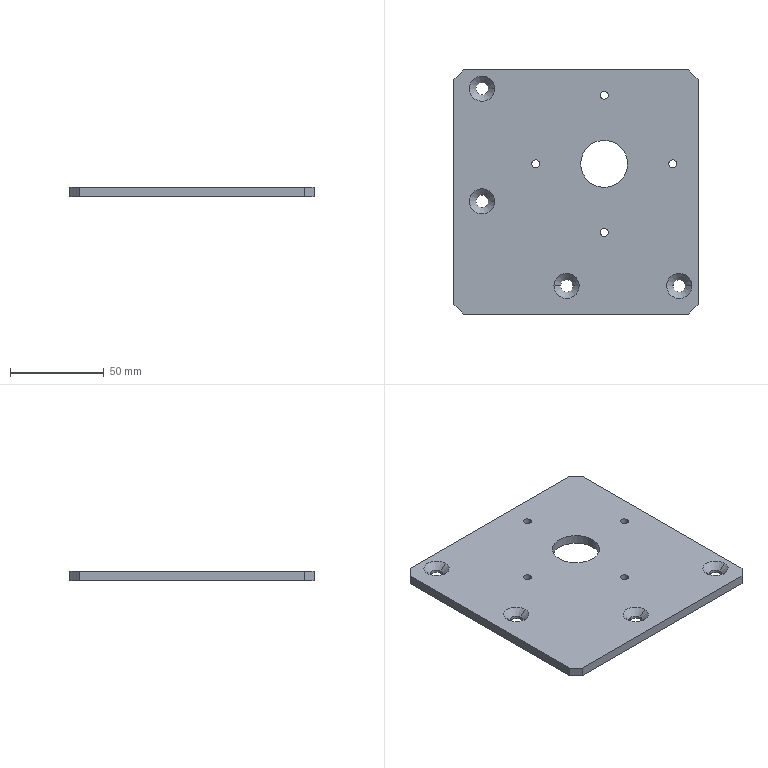Part | SolidWorks | features BaseBody 1 | 1 solid | 36 faces | box 130 x 130 x 5 mm | volume 80182 mm3 | cylinder 18 | plane 10 | cone 8 | commonest cylinder face diameters 4.2 x8 6.6 x8 25 x2
STEP:
#1=CARTESIAN_POINT('',(114.4,80.,0.));
#2=VERTEX_POINT('',#1);
#3=CARTESIAN_POINT('',(118.6,80.,0.));
#4=VERTEX_POINT('',#3);
#5=CARTESIAN_POINT('',(116.5,80.,0.));
#6=DIRECTION('',(0.,0.,1.));
#7=DIRECTION('',(1.,0.,0.));
#8=AXIS2_PLACEMENT_3D('',#5,#6,#7);
#9=CIRCLE('',#8,2.1);
#10=EDGE_CURVE('',#2,#4,#9,.T.);
#11=ORIENTED_EDGE('',*,*,#10,.F.);
#12=CARTESIAN_POINT('',(114.4,80.,5.));
#13=VERTEX_POINT('',#12);
#14=CARTESIAN_POINT('',(114.4,80.,5.));
#15=DIRECTION('',(0.,0.,1.));
#16=VECTOR('',#15,1000.);
#17=LINE('',#14,#16);
#18=EDGE_CURVE('',#2,#13,#17,.T.);
#19=ORIENTED_EDGE('',*,*,#18,.T.);
#20=CARTESIAN_POINT('',(118.6,80.,5.));
#21=VERTEX_POINT('',#20);
#22=CARTESIAN_POINT('',(116.5,80.,5.));
#23=DIRECTION('',(0.,0.,1.));
#24=DIRECTION('',(1.,0.,0.));
#25=AXIS2_PLACEMENT_3D('',#22,#23,#24);
#26=CIRCLE('',#25,2.1);
#27=EDGE_CURVE('',#13,#21,#26,.T.);
#28=ORIENTED_EDGE('',*,*,#27,.T.);
#29=CARTESIAN_POINT('',(118.6,80.,5.));
#30=DIRECTION('',(0.,0.,1.));
#31=VECTOR('',#30,1000.);
#32=LINE('',#29,#31);
#33=EDGE_CURVE('',#4,#21,#32,.T.);
#34=ORIENTED_EDGE('',*,*,#33,.F.);
#35=EDGE_LOOP('',(#11,#19,#28,#34));
#36=FACE_OUTER_BOUND('',#35,.T.);
#37=CARTESIAN_POINT('',(116.5,80.,5.));
#38=DIRECTION('',(0.,0.,1.));
#39=DIRECTION('',(1.,0.,0.));
#40=AXIS2_PLACEMENT_3D('',#37,#38,#39);
#41=CYLINDRICAL_SURFACE('',#40,2.1);
#42=ADVANCED_FACE('',(#36),#41,.F.);
#43=CARTESIAN_POINT('',(77.9,43.5,0.));
#44=VERTEX_POINT('',#43);
#45=CARTESIAN_POINT('',(82.1,43.5,0.));
#46=VERTEX_POINT('',#45);
#47=CARTESIAN_POINT('',(80.,43.5,0.));
#48=DIRECTION('',(0.,0.,1.));
#49=DIRECTION('',(1.,0.,0.));
#50=AXIS2_PLACEMENT_3D('',#47,#48,#49);
#51=CIRCLE('',#50,2.1);
#52=EDGE_CURVE('',#44,#46,#51,.T.);
#53=ORIENTED_EDGE('',*,*,#52,.F.);
#54=CARTESIAN_POINT('',(77.9,43.5,5.));
#55=VERTEX_POINT('',#54);
#56=CARTESIAN_POINT('',(77.9,43.5,5.));
#57=DIRECTION('',(0.,0.,1.));
#58=VECTOR('',#57,1000.);
#59=LINE('',#56,#58);
#60=EDGE_CURVE('',#44,#55,#59,.T.);
#61=ORIENTED_EDGE('',*,*,#60,.T.);
#62=CARTESIAN_POINT('',(82.1,43.5,5.));
#63=VERTEX_POINT('',#62);
#64=CARTESIAN_POINT('',(80.,43.5,5.));
#65=DIRECTION('',(0.,0.,1.));
#66=DIRECTION('',(1.,0.,0.));
#67=AXIS2_PLACEMENT_3D('',#64,#65,#66);
#68=CIRCLE('',#67,2.1);
#69=EDGE_CURVE('',#55,#63,#68,.T.);
#70=ORIENTED_EDGE('',*,*,#69,.T.);
#71=CARTESIAN_POINT('',(82.1,43.5,5.));
#72=DIRECTION('',(0.,0.,1.));
#73=VECTOR('',#72,1000.);
#74=LINE('',#71,#73);
#75=EDGE_CURVE('',#46,#63,#74,.T.);
#76=ORIENTED_EDGE('',*,*,#75,.F.);
#77=EDGE_LOOP('',(#53,#61,#70,#76));
#78=FACE_OUTER_BOUND('',#77,.T.);
#79=CARTESIAN_POINT('',(80.,43.5,5.));
#80=DIRECTION('',(0.,0.,1.));
#81=DIRECTION('',(1.,0.,0.));
#82=AXIS2_PLACEMENT_3D('',#79,#80,#81);
#83=CYLINDRICAL_SURFACE('',#82,2.1);
#84=ADVANCED_FACE('',(#78),#83,.F.);
#85=CARTESIAN_POINT('',(41.4,80.,0.));
#86=VERTEX_POINT('',#85);
#87=CARTESIAN_POINT('',(45.6,80.,0.));
#88=VERTEX_POINT('',#87);
#89=CARTESIAN_POINT('',(43.5,80.,0.));
#90=DIRECTION('',(0.,0.,1.));
#91=DIRECTION('',(1.,0.,0.));
#92=AXIS2_PLACEMENT_3D('',#89,#90,#91);
#93=CIRCLE('',#92,2.1);
#94=EDGE_CURVE('',#86,#88,#93,.T.);
#95=ORIENTED_EDGE('',*,*,#94,.F.);
#96=CARTESIAN_POINT('',(41.4,80.,5.));
#97=VERTEX_POINT('',#96);
#98=CARTESIAN_POINT('',(41.4,80.,5.));
#99=DIRECTION('',(0.,0.,1.));
#100=VECTOR('',#99,1000.);
#101=LINE('',#98,#100);
#102=EDGE_CURVE('',#86,#97,#101,.T.);
#103=ORIENTED_EDGE('',*,*,#102,.T.);
#104=CARTESIAN_POINT('',(45.6,80.,5.));
#105=VERTEX_POINT('',#104);
#106=CARTESIAN_POINT('',(43.5,80.,5.));
#107=DIRECTION('',(0.,0.,1.));
#108=DIRECTION('',(1.,0.,0.));
#109=AXIS2_PLACEMENT_3D('',#106,#107,#108);
#110=CIRCLE('',#109,2.1);
#111=EDGE_CURVE('',#97,#105,#110,.T.);
#112=ORIENTED_EDGE('',*,*,#111,.T.);
#113=CARTESIAN_POINT('',(45.6,80.,5.));
#114=DIRECTION('',(0.,0.,1.));
#115=VECTOR('',#114,1000.);
#116=LINE('',#113,#115);
#117=EDGE_CURVE('',#88,#105,#116,.T.);
#118=ORIENTED_EDGE('',*,*,#117,.F.);
#119=EDGE_LOOP('',(#95,#103,#112,#118));
#120=FACE_OUTER_BOUND('',#119,.T.);
#121=CARTESIAN_POINT('',(43.5,80.,5.));
#122=DIRECTION('',(0.,0.,1.));
#123=DIRECTION('',(1.,0.,0.));
#124=AXIS2_PLACEMENT_3D('',#121,#122,#123);
#125=CYLINDRICAL_SURFACE('',#124,2.1);
#126=ADVANCED_FACE('',(#120),#125,.F.);
#127=CARTESIAN_POINT('',(77.9,116.5,0.));
#128=VERTEX_POINT('',#127);
#129=CARTESIAN_POINT('',(82.1,116.5,0.));
#130=VERTEX_POINT('',#129);
#131=CARTESIAN_POINT('',(80.,116.5,0.));
#132=DIRECTION('',(0.,0.,1.));
#133=DIRECTION('',(1.,0.,0.));
#134=AXIS2_PLACEMENT_3D('',#131,#132,#133);
#135=CIRCLE('',#134,2.1);
#136=EDGE_CURVE('',#128,#130,#135,.T.);
#137=ORIENTED_EDGE('',*,*,#136,.F.);
#138=CARTESIAN_POINT('',(77.9,116.5,5.));
#139=VERTEX_POINT('',#138);
#140=CARTESIAN_POINT('',(77.9,116.5,5.));
#141=DIRECTION('',(0.,0.,1.));
#142=VECTOR('',#141,1000.);
#143=LINE('',#140,#142);
#144=EDGE_CURVE('',#128,#139,#143,.T.);
#145=ORIENTED_EDGE('',*,*,#144,.T.);
#146=CARTESIAN_POINT('',(82.1,116.5,5.));
#147=VERTEX_POINT('',#146);
#148=CARTESIAN_POINT('',(80.,116.5,5.));
#149=DIRECTION('',(0.,0.,1.));
#150=DIRECTION('',(1.,0.,0.));
#151=AXIS2_PLACEMENT_3D('',#148,#149,#150);
#152=CIRCLE('',#151,2.1);
#153=EDGE_CURVE('',#139,#147,#152,.T.);
#154=ORIENTED_EDGE('',*,*,#153,.T.);
#155=CARTESIAN_POINT('',(82.1,116.5,5.));
#156=DIRECTION('',(0.,0.,1.));
#157=VECTOR('',#156,1000.);
#158=LINE('',#155,#157);
#159=EDGE_CURVE('',#130,#147,#158,.T.);
#160=ORIENTED_EDGE('',*,*,#159,.F.);
#161=EDGE_LOOP('',(#137,#145,#154,#160));
#162=FACE_OUTER_BOUND('',#161,.T.);
#163=CARTESIAN_POINT('',(80.,116.5,5.));
#164=DIRECTION('',(0.,0.,1.));
#165=DIRECTION('',(1.,0.,0.));
#166=AXIS2_PLACEMENT_3D('',#163,#164,#165);
#167=CYLINDRICAL_SURFACE('',#166,2.1);
#168=ADVANCED_FACE('',(#162),#167,.F.);
#169=CARTESIAN_POINT('',(67.5,80.,0.));
#170=VERTEX_POINT('',#169);
#171=CARTESIAN_POINT('',(92.5,80.,0.));
#172=VERTEX_POINT('',#171);
#173=CARTESIAN_POINT('',(80.,80.,0.));
#174=DIRECTION('',(0.,0.,1.));
#175=DIRECTION('',(1.,0.,0.));
#176=AXIS2_PLACEMENT_3D('',#173,#174,#175);
#177=CIRCLE('',#176,12.5);
#178=EDGE_CURVE('',#170,#172,#177,.T.);
#179=ORIENTED_EDGE('',*,*,#178,.F.);
#180=CARTESIAN_POINT('',(67.5,80.,5.));
#181=VERTEX_POINT('',#180);
#182=CARTESIAN_POINT('',(67.5,80.,0.));
#183=DIRECTION('',(0.,0.,1.));
#184=VECTOR('',#183,1000.);
#185=LINE('',#182,#184);
#186=EDGE_CURVE('',#170,#181,#185,.T.);
#187=ORIENTED_EDGE('',*,*,#186,.T.);
#188=CARTESIAN_POINT('',(92.5,80.,5.));
#189=VERTEX_POINT('',#188);
#190=CARTESIAN_POINT('',(80.,80.,5.));
#191=DIRECTION('',(0.,0.,1.));
#192=DIRECTION('',(1.,0.,0.));
#193=AXIS2_PLACEMENT_3D('',#190,#191,#192);
#194=CIRCLE('',#193,12.5);
#195=EDGE_CURVE('',#181,#189,#194,.T.);
#196=ORIENTED_EDGE('',*,*,#195,.T.);
#197=CARTESIAN_POINT('',(92.5,80.,0.));
#198=DIRECTION('',(0.,0.,1.));
#199=VECTOR('',#198,1000.);
#200=LINE('',#197,#199);
#201=EDGE_CURVE('',#172,#189,#200,.T.);
#202=ORIENTED_EDGE('',*,*,#201,.F.);
#203=EDGE_LOOP('',(#179,#187,#196,#202));
#204=FACE_OUTER_BOUND('',#203,.T.);
#205=CARTESIAN_POINT('',(80.,80.,0.));
#206=DIRECTION('',(0.,0.,1.));
#207=DIRECTION('',(1.,0.,0.));
#208=AXIS2_PLACEMENT_3D('',#205,#206,#207);
#209=CYLINDRICAL_SURFACE('',#208,12.5);
#210=ADVANCED_FACE('',(#204),#209,.F.);
#211=CARTESIAN_POINT('',(11.7,60.,1.58));
#212=VERTEX_POINT('',#211);
#213=CARTESIAN_POINT('',(18.3,60.,1.58));
#214=VERTEX_POINT('',#213);
#215=CARTESIAN_POINT('',(15.,60.,1.58));
#216=DIRECTION('',(0.,0.,1.));
#217=DIRECTION('',(1.,0.,0.));
#218=AXIS2_PLACEMENT_3D('',#215,#216,#217);
#219=CIRCLE('',#218,3.3);
#220=EDGE_CURVE('',#212,#214,#219,.T.);
#221=ORIENTED_EDGE('',*,*,#220,.F.);
#222=CARTESIAN_POINT('',(8.28,60.,5.));
#223=VERTEX_POINT('',#222);
#224=CARTESIAN_POINT('',(8.28,60.,5.));
#225=DIRECTION('',(-0.7071,0.,0.7071));
#226=VECTOR('',#225,1000.);
#227=LINE('',#224,#226);
#228=EDGE_CURVE('',#212,#223,#227,.T.);
#229=ORIENTED_EDGE('',*,*,#228,.T.);
#230=CARTESIAN_POINT('',(21.72,60.,5.));
#231=VERTEX_POINT('',#230);
#232=CARTESIAN_POINT('',(15.,60.,5.));
#233=DIRECTION('',(0.,0.,1.));
#234=DIRECTION('',(1.,0.,0.));
#235=AXIS2_PLACEMENT_3D('',#232,#233,#234);
#236=CIRCLE('',#235,6.72);
#237=EDGE_CURVE('',#223,#231,#236,.T.);
#238=ORIENTED_EDGE('',*,*,#237,.T.);
#239=CARTESIAN_POINT('',(21.72,60.,5.));
#240=DIRECTION('',(0.7071,0.,0.7071));
#241=VECTOR('',#240,1000.);
#242=LINE('',#239,#241);
#243=EDGE_CURVE('',#214,#231,#242,.T.);
#244=ORIENTED_EDGE('',*,*,#243,.F.);
#245=EDGE_LOOP('',(#221,#229,#238,#244));
#246=FACE_OUTER_BOUND('',#245,.T.);
#247=CARTESIAN_POINT('',(15.,60.,5.));
#248=DIRECTION('',(0.,0.,1.));
#249=DIRECTION('',(1.,0.,0.));
#250=AXIS2_PLACEMENT_3D('',#247,#248,#249);
#251=CONICAL_SURFACE('',#250,6.72,0.7854);
#252=ADVANCED_FACE('',(#246),#251,.F.);
#253=CARTESIAN_POINT('',(11.7,60.,0.));
#254=VERTEX_POINT('',#253);
#255=CARTESIAN_POINT('',(18.3,60.,0.));
#256=VERTEX_POINT('',#255);
#257=CARTESIAN_POINT('',(15.,60.,0.));
#258=DIRECTION('',(0.,0.,1.));
#259=DIRECTION('',(1.,0.,0.));
#260=AXIS2_PLACEMENT_3D('',#257,#258,#259);
#261=CIRCLE('',#260,3.3);
#262=EDGE_CURVE('',#254,#256,#261,.T.);
#263=ORIENTED_EDGE('',*,*,#262,.F.);
#264=CARTESIAN_POINT('',(11.7,60.,5.));
#265=DIRECTION('',(0.,0.,1.));
#266=VECTOR('',#265,1000.);
#267=LINE('',#264,#266);
#268=EDGE_CURVE('',#254,#212,#267,.T.);
#269=ORIENTED_EDGE('',*,*,#268,.T.);
#270=ORIENTED_EDGE('',*,*,#220,.T.);
#271=CARTESIAN_POINT('',(18.3,60.,5.));
#272=DIRECTION('',(0.,0.,1.));
#273=VECTOR('',#272,1000.);
#274=LINE('',#271,#273);
#275=EDGE_CURVE('',#256,#214,#274,.T.);
#276=ORIENTED_EDGE('',*,*,#275,.F.);
#277=EDGE_LOOP('',(#263,#269,#270,#276));
#278=FACE_OUTER_BOUND('',#277,.T.);
#279=CARTESIAN_POINT('',(15.,60.,5.));
#280=DIRECTION('',(0.,0.,1.));
#281=DIRECTION('',(1.,0.,0.));
#282=AXIS2_PLACEMENT_3D('',#279,#280,#281);
#283=CYLINDRICAL_SURFACE('',#282,3.3);
#284=ADVANCED_FACE('',(#278),#283,.F.);
#285=CARTESIAN_POINT('',(11.7,120.,1.58));
#286=VERTEX_POINT('',#285);
#287=CARTESIAN_POINT('',(18.3,120.,1.58));
#288=VERTEX_POINT('',#287);
#289=CARTESIAN_POINT('',(15.,120.,1.58));
#290=DIRECTION('',(0.,0.,1.));
#291=DIRECTION('',(1.,0.,0.));
#292=AXIS2_PLACEMENT_3D('',#289,#290,#291);
#293=CIRCLE('',#292,3.3);
#294=EDGE_CURVE('',#286,#288,#293,.T.);
#295=ORIENTED_EDGE('',*,*,#294,.F.);
#296=CARTESIAN_POINT('',(8.28,120.,5.));
#297=VERTEX_POINT('',#296);
#298=CARTESIAN_POINT('',(8.28,120.,5.));
#299=DIRECTION('',(-0.7071,0.,0.7071));
#300=VECTOR('',#299,1000.);
#301=LINE('',#298,#300);
#302=EDGE_CURVE('',#286,#297,#301,.T.);
#303=ORIENTED_EDGE('',*,*,#302,.T.);
#304=CARTESIAN_POINT('',(21.72,120.,5.));
#305=VERTEX_POINT('',#304);
#306=CARTESIAN_POINT('',(15.,120.,5.));
#307=DIRECTION('',(0.,0.,1.));
#308=DIRECTION('',(1.,0.,0.));
#309=AXIS2_PLACEMENT_3D('',#306,#307,#308);
#310=CIRCLE('',#309,6.72);
#311=EDGE_CURVE('',#297,#305,#310,.T.);
#312=ORIENTED_EDGE('',*,*,#311,.T.);
#313=CARTESIAN_POINT('',(21.72,120.,5.));
#314=DIRECTION('',(0.7071,0.,0.7071));
#315=VECTOR('',#314,1000.);
#316=LINE('',#313,#315);
#317=EDGE_CURVE('',#288,#305,#316,.T.);
#318=ORIENTED_EDGE('',*,*,#317,.F.);
#319=EDGE_LOOP('',(#295,#303,#312,#318));
#320=FACE_OUTER_BOUND('',#319,.T.);
#321=CARTESIAN_POINT('',(15.,120.,5.));
#322=DIRECTION('',(0.,0.,1.));
#323=DIRECTION('',(1.,0.,0.));
#324=AXIS2_PLACEMENT_3D('',#321,#322,#323);
#325=CONICAL_SURFACE('',#324,6.72,0.7854);
#326=ADVANCED_FACE('',(#320),#325,.F.);
#327=CARTESIAN_POINT('',(11.7,120.,0.));
#328=VERTEX_POINT('',#327);
#329=CARTESIAN_POINT('',(18.3,120.,0.));
#330=VERTEX_POINT('',#329);
#331=CARTESIAN_POINT('',(15.,120.,0.));
#332=DIRECTION('',(0.,0.,1.));
#333=DIRECTION('',(1.,0.,0.));
#334=AXIS2_PLACEMENT_3D('',#331,#332,#333);
#335=CIRCLE('',#334,3.3);
#336=EDGE_CURVE('',#328,#330,#335,.T.);
#337=ORIENTED_EDGE('',*,*,#336,.F.);
#338=CARTESIAN_POINT('',(11.7,120.,5.));
#339=DIRECTION('',(0.,0.,1.));
#340=VECTOR('',#339,1000.);
#341=LINE('',#338,#340);
#342=EDGE_CURVE('',#328,#286,#341,.T.);
#343=ORIENTED_EDGE('',*,*,#342,.T.);
#344=ORIENTED_EDGE('',*,*,#294,.T.);
#345=CARTESIAN_POINT('',(18.3,120.,5.));
#346=DIRECTION('',(0.,0.,1.));
#347=VECTOR('',#346,1000.);
#348=LINE('',#345,#347);
#349=EDGE_CURVE('',#330,#288,#348,.T.);
#350=ORIENTED_EDGE('',*,*,#349,.F.);
#351=EDGE_LOOP('',(#337,#343,#344,#350));
#352=FACE_OUTER_BOUND('',#351,.T.);
#353=CARTESIAN_POINT('',(15.,120.,5.));
#354=DIRECTION('',(0.,0.,1.));
#355=DIRECTION('',(1.,0.,0.));
#356=AXIS2_PLACEMENT_3D('',#353,#354,#355);
#357=CYLINDRICAL_SURFACE('',#356,3.3);
#358=ADVANCED_FACE('',(#352),#357,.F.);
#359=CARTESIAN_POINT('',(56.7,15.,1.58));
#360=VERTEX_POINT('',#359);
#361=CARTESIAN_POINT('',(63.3,15.,1.58));
#362=VERTEX_POINT('',#361);
#363=CARTESIAN_POINT('',(60.,15.,1.58));
#364=DIRECTION('',(0.,0.,1.));
#365=DIRECTION('',(1.,0.,0.));
#366=AXIS2_PLACEMENT_3D('',#363,#364,#365);
#367=CIRCLE('',#366,3.3);
#368=EDGE_CURVE('',#360,#362,#367,.T.);
#369=ORIENTED_EDGE('',*,*,#368,.F.);
#370=CARTESIAN_POINT('',(53.28,15.,5.));
#371=VERTEX_POINT('',#370);
#372=CARTESIAN_POINT('',(53.28,15.,5.));
#373=DIRECTION('',(-0.7071,0.,0.7071));
#374=VECTOR('',#373,1000.);
#375=LINE('',#372,#374);
#376=EDGE_CURVE('',#360,#371,#375,.T.);
#377=ORIENTED_EDGE('',*,*,#376,.T.);
#378=CARTESIAN_POINT('',(66.72,15.,5.));
#379=VERTEX_POINT('',#378);
#380=CARTESIAN_POINT('',(60.,15.,5.));
#381=DIRECTION('',(0.,0.,1.));
#382=DIRECTION('',(1.,0.,0.));
#383=AXIS2_PLACEMENT_3D('',#380,#381,#382);
#384=CIRCLE('',#383,6.72);
#385=EDGE_CURVE('',#371,#379,#384,.T.);
#386=ORIENTED_EDGE('',*,*,#385,.T.);
#387=CARTESIAN_POINT('',(66.72,15.,5.));
#388=DIRECTION('',(0.7071,0.,0.7071));
#389=VECTOR('',#388,1000.);
#390=LINE('',#387,#389);
#391=EDGE_CURVE('',#362,#379,#390,.T.);
#392=ORIENTED_EDGE('',*,*,#391,.F.);
#393=EDGE_LOOP('',(#369,#377,#386,#392));
#394=FACE_OUTER_BOUND('',#393,.T.);
#395=CARTESIAN_POINT('',(60.,15.,5.));
#396=DIRECTION('',(0.,0.,1.));
#397=DIRECTION('',(1.,0.,0.));
#398=AXIS2_PLACEMENT_3D('',#395,#396,#397);
#399=CONICAL_SURFACE('',#398,6.72,0.7854);
#400=ADVANCED_FACE('',(#394),#399,.F.);
#401=CARTESIAN_POINT('',(56.7,15.,0.));
#402=VERTEX_POINT('',#401);
#403=CARTESIAN_POINT('',(63.3,15.,0.));
#404=VERTEX_POINT('',#403);
#405=CARTESIAN_POINT('',(60.,15.,0.));
#406=DIRECTION('',(0.,0.,1.));
#407=DIRECTION('',(1.,0.,0.));
#408=AXIS2_PLACEMENT_3D('',#405,#406,#407);
#409=CIRCLE('',#408,3.3);
#410=EDGE_CURVE('',#402,#404,#409,.T.);
#411=ORIENTED_EDGE('',*,*,#410,.F.);
#412=CARTESIAN_POINT('',(56.7,15.,5.));
#413=DIRECTION('',(0.,0.,1.));
#414=VECTOR('',#413,1000.);
#415=LINE('',#412,#414);
#416=EDGE_CURVE('',#402,#360,#415,.T.);
#417=ORIENTED_EDGE('',*,*,#416,.T.);
#418=ORIENTED_EDGE('',*,*,#368,.T.);
#419=CARTESIAN_POINT('',(63.3,15.,5.));
#420=DIRECTION('',(0.,0.,1.));
#421=VECTOR('',#420,1000.);
#422=LINE('',#419,#421);
#423=EDGE_CURVE('',#404,#362,#422,.T.);
#424=ORIENTED_EDGE('',*,*,#423,.F.);
#425=EDGE_LOOP('',(#411,#417,#418,#424));
#426=FACE_OUTER_BOUND('',#425,.T.);
#427=CARTESIAN_POINT('',(60.,15.,5.));
#428=DIRECTION('',(0.,0.,1.));
#429=DIRECTION('',(1.,0.,0.));
#430=AXIS2_PLACEMENT_3D('',#427,#428,#429);
#431=CYLINDRICAL_SURFACE('',#430,3.3);
#432=ADVANCED_FACE('',(#426),#431,.F.);
#433=CARTESIAN_POINT('',(116.7,15.,1.58));
#434=VERTEX_POINT('',#433);
#435=CARTESIAN_POINT('',(123.3,15.,1.58));
#436=VERTEX_POINT('',#435);
#437=CARTESIAN_POINT('',(120.,15.,1.58));
#438=DIRECTION('',(0.,0.,1.));
#439=DIRECTION('',(1.,0.,0.));
#440=AXIS2_PLACEMENT_3D('',#437,#438,#439);
#441=CIRCLE('',#440,3.3);
#442=EDGE_CURVE('',#434,#436,#441,.T.);
#443=ORIENTED_EDGE('',*,*,#442,.F.);
#444=CARTESIAN_POINT('',(113.28,15.,5.));
#445=VERTEX_POINT('',#444);
#446=CARTESIAN_POINT('',(113.28,15.,5.));
#447=DIRECTION('',(-0.7071,0.,0.7071));
#448=VECTOR('',#447,1000.);
#449=LINE('',#446,#448);
#450=EDGE_CURVE('',#434,#445,#449,.T.);
#451=ORIENTED_EDGE('',*,*,#450,.T.);
#452=CARTESIAN_POINT('',(126.72,15.,5.));
#453=VERTEX_POINT('',#452);
#454=CARTESIAN_POINT('',(120.,15.,5.));
#455=DIRECTION('',(0.,0.,1.));
#456=DIRECTION('',(1.,0.,0.));
#457=AXIS2_PLACEMENT_3D('',#454,#455,#456);
#458=CIRCLE('',#457,6.72);
#459=EDGE_CURVE('',#445,#453,#458,.T.);
#460=ORIENTED_EDGE('',*,*,#459,.T.);
#461=CARTESIAN_POINT('',(126.72,15.,5.));
#462=DIRECTION('',(0.7071,0.,0.7071));
#463=VECTOR('',#462,1000.);
#464=LINE('',#461,#463);
#465=EDGE_CURVE('',#436,#453,#464,.T.);
#466=ORIENTED_EDGE('',*,*,#465,.F.);
#467=EDGE_LOOP('',(#443,#451,#460,#466));
#468=FACE_OUTER_BOUND('',#467,.T.);
#469=CARTESIAN_POINT('',(120.,15.,5.));
#470=DIRECTION('',(0.,0.,1.));
#471=DIRECTION('',(1.,0.,0.));
#472=AXIS2_PLACEMENT_3D('',#469,#470,#471);
#473=CONICAL_SURFACE('',#472,6.72,0.7854);
#474=ADVANCED_FACE('',(#468),#473,.F.);
#475=CARTESIAN_POINT('',(116.7,15.,0.));
#476=VERTEX_POINT('',#475);
#477=CARTESIAN_POINT('',(123.3,15.,0.));
#478=VERTEX_POINT('',#477);
#479=CARTESIAN_POINT('',(120.,15.,0.));
#480=DIRECTION('',(0.,0.,1.));
#481=DIRECTION('',(1.,0.,0.));
#482=AXIS2_PLACEMENT_3D('',#479,#480,#481);
#483=CIRCLE('',#482,3.3);
#484=EDGE_CURVE('',#476,#478,#483,.T.);
#485=ORIENTED_EDGE('',*,*,#484,.F.);
#486=CARTESIAN_POINT('',(116.7,15.,5.));
#487=DIRECTION('',(0.,0.,1.));
#488=VECTOR('',#487,1000.);
#489=LINE('',#486,#488);
#490=EDGE_CURVE('',#476,#434,#489,.T.);
#491=ORIENTED_EDGE('',*,*,#490,.T.);
#492=ORIENTED_EDGE('',*,*,#442,.T.);
#493=CARTESIAN_POINT('',(123.3,15.,5.));
#494=DIRECTION('',(0.,0.,1.));
#495=VECTOR('',#494,1000.);
#496=LINE('',#493,#495);
#497=EDGE_CURVE('',#478,#436,#496,.T.);
#498=ORIENTED_EDGE('',*,*,#497,.F.);
#499=EDGE_LOOP('',(#485,#491,#492,#498));
#500=FACE_OUTER_BOUND('',#499,.T.);
#501=CARTESIAN_POINT('',(120.,15.,5.));
#502=DIRECTION('',(0.,0.,1.));
#503=DIRECTION('',(1.,0.,0.));
#504=AXIS2_PLACEMENT_3D('',#501,#502,#503);
#505=CYLINDRICAL_SURFACE('',#504,3.3);
#506=ADVANCED_FACE('',(#500),#505,.F.);
#507=CARTESIAN_POINT('',(130.,125.,5.));
#508=VERTEX_POINT('',#507);
#509=CARTESIAN_POINT('',(125.,130.,5.));
#510=VERTEX_POINT('',#509);
#511=CARTESIAN_POINT('',(125.,130.,5.));
#512=DIRECTION('',(-0.7071,0.7071,0.));
#513=VECTOR('',#512,1000.);
#514=LINE('',#511,#513);
#515=EDGE_CURVE('',#508,#510,#514,.T.);
#516=ORIENTED_EDGE('',*,*,#515,.F.);
#517=CARTESIAN_POINT('',(130.,125.,0.));
#518=VERTEX_POINT('',#517);
#519=CARTESIAN_POINT('',(130.,125.,5.));
#520=DIRECTION('',(0.,0.,1.));
#521=VECTOR('',#520,1000.);
#522=LINE('',#519,#521);
#523=EDGE_CURVE('',#518,#508,#522,.T.);
#524=ORIENTED_EDGE('',*,*,#523,.F.);
#525=CARTESIAN_POINT('',(125.,130.,0.));
#526=VERTEX_POINT('',#525);
#527=CARTESIAN_POINT('',(127.5,127.5,0.));
#528=DIRECTION('',(0.7071,-0.7071,0.));
#529=VECTOR('',#528,1000.);
#530=LINE('',#527,#529);
#531=EDGE_CURVE('',#526,#518,#530,.T.);
#532=ORIENTED_EDGE('',*,*,#531,.F.);
#533=CARTESIAN_POINT('',(125.,130.,5.));
#534=DIRECTION('',(0.,0.,-1.));
#535=VECTOR('',#534,1000.);
#536=LINE('',#533,#535);
#537=EDGE_CURVE('',#510,#526,#536,.T.);
#538=ORIENTED_EDGE('',*,*,#537,.F.);
#539=EDGE_LOOP('',(#516,#524,#532,#538));
#540=FACE_OUTER_BOUND('',#539,.T.);
#541=CARTESIAN_POINT('',(125.,130.,5.));
#542=DIRECTION('',(-0.7071,-0.7071,0.));
#543=DIRECTION('',(-0.7071,0.7071,0.));
#544=AXIS2_PLACEMENT_3D('',#541,#542,#543);
#545=PLANE('',#544);
#546=ADVANCED_FACE('',(#540),#545,.F.);
#547=CARTESIAN_POINT('',(125.,0.,5.));
#548=VERTEX_POINT('',#547);
#549=CARTESIAN_POINT('',(130.,5.,5.));
#550=VERTEX_POINT('',#549);
#551=CARTESIAN_POINT('',(130.,5.,5.));
#552=DIRECTION('',(0.7071,0.7071,0.));
#553=VECTOR('',#552,1000.);
#554=LINE('',#551,#553);
#555=EDGE_CURVE('',#548,#550,#554,.T.);
#556=ORIENTED_EDGE('',*,*,#555,.F.);
#557=CARTESIAN_POINT('',(125.,0.,0.));
#558=VERTEX_POINT('',#557);
#559=CARTESIAN_POINT('',(125.,0.,5.));
#560=DIRECTION('',(0.,0.,1.));
#561=VECTOR('',#560,1000.);
#562=LINE('',#559,#561);
#563=EDGE_CURVE('',#558,#548,#562,.T.);
#564=ORIENTED_EDGE('',*,*,#563,.F.);
#565=CARTESIAN_POINT('',(130.,5.,0.));
#566=VERTEX_POINT('',#565);
#567=CARTESIAN_POINT('',(62.5,-62.5,0.));
#568=DIRECTION('',(-0.7071,-0.7071,0.));
#569=VECTOR('',#568,1000.);
#570=LINE('',#567,#569);
#571=EDGE_CURVE('',#566,#558,#570,.T.);
#572=ORIENTED_EDGE('',*,*,#571,.F.);
#573=CARTESIAN_POINT('',(130.,5.,5.));
#574=DIRECTION('',(0.,0.,-1.));
#575=VECTOR('',#574,1000.);
#576=LINE('',#573,#575);
#577=EDGE_CURVE('',#550,#566,#576,.T.);
#578=ORIENTED_EDGE('',*,*,#577,.F.);
#579=EDGE_LOOP('',(#556,#564,#572,#578));
#580=FACE_OUTER_BOUND('',#579,.T.);
#581=CARTESIAN_POINT('',(130.,5.,5.));
#582=DIRECTION('',(-0.7071,0.7071,0.));
#583=DIRECTION('',(0.,0.,1.));
#584=AXIS2_PLACEMENT_3D('',#581,#582,#583);
#585=PLANE('',#584);
#586=ADVANCED_FACE('',(#580),#585,.F.);
#587=CARTESIAN_POINT('',(0.,5.,5.));
#588=VERTEX_POINT('',#587);
#589=CARTESIAN_POINT('',(5.,0.,5.));
#590=VERTEX_POINT('',#589);
#591=CARTESIAN_POINT('',(5.,0.,5.));
#592=DIRECTION('',(0.7071,-0.7071,0.));
#593=VECTOR('',#592,1000.);
#594=LINE('',#591,#593);
#595=EDGE_CURVE('',#588,#590,#594,.T.);
#596=ORIENTED_EDGE('',*,*,#595,.F.);
#597=CARTESIAN_POINT('',(0.,5.,0.));
#598=VERTEX_POINT('',#597);
#599=CARTESIAN_POINT('',(0.,5.,5.));
#600=DIRECTION('',(0.,0.,1.));
#601=VECTOR('',#600,1000.);
#602=LINE('',#599,#601);
#603=EDGE_CURVE('',#598,#588,#602,.T.);
#604=ORIENTED_EDGE('',*,*,#603,.F.);
#605=CARTESIAN_POINT('',(5.,0.,0.));
#606=VERTEX_POINT('',#605);
#607=CARTESIAN_POINT('',(2.5,2.5,0.));
#608=DIRECTION('',(-0.7071,0.7071,0.));
#609=VECTOR('',#608,1000.);
#610=LINE('',#607,#609);
#611=EDGE_CURVE('',#606,#598,#610,.T.);
#612=ORIENTED_EDGE('',*,*,#611,.F.);
#613=CARTESIAN_POINT('',(5.,0.,5.));
#614=DIRECTION('',(0.,0.,-1.));
#615=VECTOR('',#614,1000.);
#616=LINE('',#613,#615);
#617=EDGE_CURVE('',#590,#606,#616,.T.);
#618=ORIENTED_EDGE('',*,*,#617,.F.);
#619=EDGE_LOOP('',(#596,#604,#612,#618));
#620=FACE_OUTER_BOUND('',#619,.T.);
#621=CARTESIAN_POINT('',(5.,0.,5.));
#622=DIRECTION('',(0.7071,0.7071,0.));
#623=DIRECTION('',(0.,0.,-1.));
#624=AXIS2_PLACEMENT_3D('',#621,#622,#623);
#625=PLANE('',#624);
#626=ADVANCED_FACE('',(#620),#625,.F.);
#627=CARTESIAN_POINT('',(5.,130.,5.));
#628=VERTEX_POINT('',#627);
#629=CARTESIAN_POINT('',(0.,125.,5.));
#630=VERTEX_POINT('',#629);
#631=CARTESIAN_POINT('',(0.,125.,5.));
#632=DIRECTION('',(-0.7071,-0.7071,0.));
#633=VECTOR('',#632,1000.);
#634=LINE('',#631,#633);
#635=EDGE_CURVE('',#628,#630,#634,.T.);
#636=ORIENTED_EDGE('',*,*,#635,.F.);
#637=CARTESIAN_POINT('',(5.,130.,0.));
#638=VERTEX_POINT('',#637);
#639=CARTESIAN_POINT('',(5.,130.,5.));
#640=DIRECTION('',(0.,0.,1.));
#641=VECTOR('',#640,1000.);
#642=LINE('',#639,#641);
#643=EDGE_CURVE('',#638,#628,#642,.T.);
#644=ORIENTED_EDGE('',*,*,#643,.F.);
#645=CARTESIAN_POINT('',(0.,125.,0.));
#646=VERTEX_POINT('',#645);
#647=CARTESIAN_POINT('',(-62.5,62.5,0.));
#648=DIRECTION('',(0.7071,0.7071,0.));
#649=VECTOR('',#648,1000.);
#650=LINE('',#647,#649);
#651=EDGE_CURVE('',#646,#638,#650,.T.);
#652=ORIENTED_EDGE('',*,*,#651,.F.);
#653=CARTESIAN_POINT('',(0.,125.,5.));
#654=DIRECTION('',(0.,0.,-1.));
#655=VECTOR('',#654,1000.);
#656=LINE('',#653,#655);
#657=EDGE_CURVE('',#630,#646,#656,.T.);
#658=ORIENTED_EDGE('',*,*,#657,.F.);
#659=EDGE_LOOP('',(#636,#644,#652,#658));
#660=FACE_OUTER_BOUND('',#659,.T.);
#661=CARTESIAN_POINT('',(0.,125.,5.));
#662=DIRECTION('',(0.7071,-0.7071,0.));
#663=DIRECTION('',(0.,0.,-1.));
#664=AXIS2_PLACEMENT_3D('',#661,#662,#663);
#665=PLANE('',#664);
#666=ADVANCED_FACE('',(#660),#665,.F.);
#667=CARTESIAN_POINT('',(120.,15.,0.));
#668=DIRECTION('',(0.,0.,1.));
#669=DIRECTION('',(1.,0.,0.));
#670=AXIS2_PLACEMENT_3D('',#667,#668,#669);
#671=CIRCLE('',#670,3.3);
#672=EDGE_CURVE('',#478,#476,#671,.T.);
#673=ORIENTED_EDGE('',*,*,#672,.T.);
#674=ORIENTED_EDGE('',*,*,#484,.T.);
#675=EDGE_LOOP('',(#673,#674));
#676=FACE_BOUND('',#675,.T.);
#677=CARTESIAN_POINT('',(60.,15.,0.));
#678=DIRECTION('',(0.,0.,1.));
#679=DIRECTION('',(1.,0.,0.));
#680=AXIS2_PLACEMENT_3D('',#677,#678,#679);
#681=CIRCLE('',#680,3.3);
#682=EDGE_CURVE('',#404,#402,#681,.T.);
#683=ORIENTED_EDGE('',*,*,#682,.T.);
#684=ORIENTED_EDGE('',*,*,#410,.T.);
#685=EDGE_LOOP('',(#683,#684));
#686=FACE_BOUND('',#685,.T.);
#687=CARTESIAN_POINT('',(15.,120.,0.));
#688=DIRECTION('',(0.,0.,1.));
#689=DIRECTION('',(1.,0.,0.));
#690=AXIS2_PLACEMENT_3D('',#687,#688,#689);
#691=CIRCLE('',#690,3.3);
#692=EDGE_CURVE('',#330,#328,#691,.T.);
#693=ORIENTED_EDGE('',*,*,#692,.T.);
#694=ORIENTED_EDGE('',*,*,#336,.T.);
#695=EDGE_LOOP('',(#693,#694));
#696=FACE_BOUND('',#695,.T.);
#697=CARTESIAN_POINT('',(15.,60.,0.));
#698=DIRECTION('',(0.,0.,1.));
#699=DIRECTION('',(1.,0.,0.));
#700=AXIS2_PLACEMENT_3D('',#697,#698,#699);
#701=CIRCLE('',#700,3.3);
#702=EDGE_CURVE('',#256,#254,#701,.T.);
#703=ORIENTED_EDGE('',*,*,#702,.T.);
#704=ORIENTED_EDGE('',*,*,#262,.T.);
#705=EDGE_LOOP('',(#703,#704));
#706=FACE_BOUND('',#705,.T.);
#707=CARTESIAN_POINT('',(80.,80.,0.));
#708=DIRECTION('',(0.,0.,1.));
#709=DIRECTION('',(1.,0.,0.));
#710=AXIS2_PLACEMENT_3D('',#707,#708,#709);
#711=CIRCLE('',#710,12.5);
#712=EDGE_CURVE('',#172,#170,#711,.T.);
#713=ORIENTED_EDGE('',*,*,#712,.T.);
#714=ORIENTED_EDGE('',*,*,#178,.T.);
#715=EDGE_LOOP('',(#713,#714));
#716=FACE_BOUND('',#715,.T.);
#717=CARTESIAN_POINT('',(80.,116.5,0.));
#718=DIRECTION('',(0.,0.,1.));
#719=DIRECTION('',(1.,0.,0.));
#720=AXIS2_PLACEMENT_3D('',#717,#718,#719);
#721=CIRCLE('',#720,2.1);
#722=EDGE_CURVE('',#130,#128,#721,.T.);
#723=ORIENTED_EDGE('',*,*,#722,.T.);
#724=ORIENTED_EDGE('',*,*,#136,.T.);
#725=EDGE_LOOP('',(#723,#724));
#726=FACE_BOUND('',#725,.T.);
#727=CARTESIAN_POINT('',(43.5,80.,0.));
#728=DIRECTION('',(0.,0.,1.));
#729=DIRECTION('',(1.,0.,0.));
#730=AXIS2_PLACEMENT_3D('',#727,#728,#729);
#731=CIRCLE('',#730,2.1);
#732=EDGE_CURVE('',#88,#86,#731,.T.);
#733=ORIENTED_EDGE('',*,*,#732,.T.);
#734=ORIENTED_EDGE('',*,*,#94,.T.);
#735=EDGE_LOOP('',(#733,#734));
#736=FACE_BOUND('',#735,.T.);
#737=CARTESIAN_POINT('',(80.,43.5,0.));
#738=DIRECTION('',(0.,0.,1.));
#739=DIRECTION('',(1.,0.,0.));
#740=AXIS2_PLACEMENT_3D('',#737,#738,#739);
#741=CIRCLE('',#740,2.1);
#742=EDGE_CURVE('',#46,#44,#741,.T.);
#743=ORIENTED_EDGE('',*,*,#742,.T.);
#744=ORIENTED_EDGE('',*,*,#52,.T.);
#745=EDGE_LOOP('',(#743,#744));
#746=FACE_BOUND('',#745,.T.);
#747=CARTESIAN_POINT('',(116.5,80.,0.));
#748=DIRECTION('',(0.,0.,1.));
#749=DIRECTION('',(1.,0.,0.));
#750=AXIS2_PLACEMENT_3D('',#747,#748,#749);
#751=CIRCLE('',#750,2.1);
#752=EDGE_CURVE('',#4,#2,#751,.T.);
#753=ORIENTED_EDGE('',*,*,#752,.T.);
#754=ORIENTED_EDGE('',*,*,#10,.T.);
#755=EDGE_LOOP('',(#753,#754));
#756=FACE_BOUND('',#755,.T.);
#757=CARTESIAN_POINT('',(0.,0.,0.));
#758=DIRECTION('',(0.,-1.,0.));
#759=VECTOR('',#758,1000.);
#760=LINE('',#757,#759);
#761=EDGE_CURVE('',#646,#598,#760,.T.);
#762=ORIENTED_EDGE('',*,*,#761,.F.);
#763=ORIENTED_EDGE('',*,*,#651,.T.);
#764=CARTESIAN_POINT('',(0.,130.,0.));
#765=DIRECTION('',(-1.,0.,0.));
#766=VECTOR('',#765,1000.);
#767=LINE('',#764,#766);
#768=EDGE_CURVE('',#526,#638,#767,.T.);
#769=ORIENTED_EDGE('',*,*,#768,.F.);
#770=ORIENTED_EDGE('',*,*,#531,.T.);
#771=CARTESIAN_POINT('',(130.,0.,0.));
#772=DIRECTION('',(0.,1.,0.));
#773=VECTOR('',#772,1000.);
#774=LINE('',#771,#773);
#775=EDGE_CURVE('',#566,#518,#774,.T.);
#776=ORIENTED_EDGE('',*,*,#775,.F.);
#777=ORIENTED_EDGE('',*,*,#571,.T.);
#778=CARTESIAN_POINT('',(0.,0.,0.));
#779=DIRECTION('',(1.,0.,0.));
#780=VECTOR('',#779,1000.);
#781=LINE('',#778,#780);
#782=EDGE_CURVE('',#606,#558,#781,.T.);
#783=ORIENTED_EDGE('',*,*,#782,.F.);
#784=ORIENTED_EDGE('',*,*,#611,.T.);
#785=EDGE_LOOP('',(#762,#763,#769,#770,#776,#777,#783,#784));
#786=FACE_OUTER_BOUND('',#785,.T.);
#787=CARTESIAN_POINT('',(0.,0.,0.));
#788=DIRECTION('',(0.,0.,-1.));
#789=DIRECTION('',(0.,-1.,0.));
#790=AXIS2_PLACEMENT_3D('',#787,#788,#789);
#791=PLANE('',#790);
#792=ADVANCED_FACE('',(#676,#686,#696,#706,#716,#726,#736,#746,#756,#786),#791,.T.);
#793=CARTESIAN_POINT('',(120.,15.,5.));
#794=DIRECTION('',(0.,0.,1.));
#795=DIRECTION('',(1.,0.,0.));
#796=AXIS2_PLACEMENT_3D('',#793,#794,#795);
#797=CIRCLE('',#796,6.72);
#798=EDGE_CURVE('',#453,#445,#797,.T.);
#799=ORIENTED_EDGE('',*,*,#798,.F.);
#800=ORIENTED_EDGE('',*,*,#459,.F.);
#801=EDGE_LOOP('',(#799,#800));
#802=FACE_BOUND('',#801,.T.);
#803=CARTESIAN_POINT('',(60.,15.,5.));
#804=DIRECTION('',(0.,0.,1.));
#805=DIRECTION('',(1.,0.,0.));
#806=AXIS2_PLACEMENT_3D('',#803,#804,#805);
#807=CIRCLE('',#806,6.72);
#808=EDGE_CURVE('',#379,#371,#807,.T.);
#809=ORIENTED_EDGE('',*,*,#808,.F.);
#810=ORIENTED_EDGE('',*,*,#385,.F.);
#811=EDGE_LOOP('',(#809,#810));
#812=FACE_BOUND('',#811,.T.);
#813=CARTESIAN_POINT('',(15.,120.,5.));
#814=DIRECTION('',(0.,0.,1.));
#815=DIRECTION('',(1.,0.,0.));
#816=AXIS2_PLACEMENT_3D('',#813,#814,#815);
#817=CIRCLE('',#816,6.72);
#818=EDGE_CURVE('',#305,#297,#817,.T.);
#819=ORIENTED_EDGE('',*,*,#818,.F.);
#820=ORIENTED_EDGE('',*,*,#311,.F.);
#821=EDGE_LOOP('',(#819,#820));
#822=FACE_BOUND('',#821,.T.);
#823=CARTESIAN_POINT('',(15.,60.,5.));
#824=DIRECTION('',(0.,0.,1.));
#825=DIRECTION('',(1.,0.,0.));
#826=AXIS2_PLACEMENT_3D('',#823,#824,#825);
#827=CIRCLE('',#826,6.72);
#828=EDGE_CURVE('',#231,#223,#827,.T.);
#829=ORIENTED_EDGE('',*,*,#828,.F.);
#830=ORIENTED_EDGE('',*,*,#237,.F.);
#831=EDGE_LOOP('',(#829,#830));
#832=FACE_BOUND('',#831,.T.);
#833=CARTESIAN_POINT('',(80.,80.,5.));
#834=DIRECTION('',(0.,0.,1.));
#835=DIRECTION('',(1.,0.,0.));
#836=AXIS2_PLACEMENT_3D('',#833,#834,#835);
#837=CIRCLE('',#836,12.5);
#838=EDGE_CURVE('',#189,#181,#837,.T.);
#839=ORIENTED_EDGE('',*,*,#838,.F.);
#840=ORIENTED_EDGE('',*,*,#195,.F.);
#841=EDGE_LOOP('',(#839,#840));
#842=FACE_BOUND('',#841,.T.);
#843=CARTESIAN_POINT('',(80.,116.5,5.));
#844=DIRECTION('',(0.,0.,1.));
#845=DIRECTION('',(1.,0.,0.));
#846=AXIS2_PLACEMENT_3D('',#843,#844,#845);
#847=CIRCLE('',#846,2.1);
#848=EDGE_CURVE('',#147,#139,#847,.T.);
#849=ORIENTED_EDGE('',*,*,#848,.F.);
#850=ORIENTED_EDGE('',*,*,#153,.F.);
#851=EDGE_LOOP('',(#849,#850));
#852=FACE_BOUND('',#851,.T.);
#853=CARTESIAN_POINT('',(43.5,80.,5.));
#854=DIRECTION('',(0.,0.,1.));
#855=DIRECTION('',(1.,0.,0.));
#856=AXIS2_PLACEMENT_3D('',#853,#854,#855);
#857=CIRCLE('',#856,2.1);
#858=EDGE_CURVE('',#105,#97,#857,.T.);
#859=ORIENTED_EDGE('',*,*,#858,.F.);
#860=ORIENTED_EDGE('',*,*,#111,.F.);
#861=EDGE_LOOP('',(#859,#860));
#862=FACE_BOUND('',#861,.T.);
#863=CARTESIAN_POINT('',(80.,43.5,5.));
#864=DIRECTION('',(0.,0.,1.));
#865=DIRECTION('',(1.,0.,0.));
#866=AXIS2_PLACEMENT_3D('',#863,#864,#865);
#867=CIRCLE('',#866,2.1);
#868=EDGE_CURVE('',#63,#55,#867,.T.);
#869=ORIENTED_EDGE('',*,*,#868,.F.);
#870=ORIENTED_EDGE('',*,*,#69,.F.);
#871=EDGE_LOOP('',(#869,#870));
#872=FACE_BOUND('',#871,.T.);
#873=CARTESIAN_POINT('',(116.5,80.,5.));
#874=DIRECTION('',(0.,0.,1.));
#875=DIRECTION('',(1.,0.,0.));
#876=AXIS2_PLACEMENT_3D('',#873,#874,#875);
#877=CIRCLE('',#876,2.1);
#878=EDGE_CURVE('',#21,#13,#877,.T.);
#879=ORIENTED_EDGE('',*,*,#878,.F.);
#880=ORIENTED_EDGE('',*,*,#27,.F.);
#881=EDGE_LOOP('',(#879,#880));
#882=FACE_BOUND('',#881,.T.);
#883=CARTESIAN_POINT('',(0.,130.,5.));
#884=DIRECTION('',(-1.,0.,0.));
#885=VECTOR('',#884,1000.);
#886=LINE('',#883,#885);
#887=EDGE_CURVE('',#510,#628,#886,.T.);
#888=ORIENTED_EDGE('',*,*,#887,.T.);
#889=ORIENTED_EDGE('',*,*,#635,.T.);
#890=CARTESIAN_POINT('',(0.,0.,5.));
#891=DIRECTION('',(0.,-1.,0.));
#892=VECTOR('',#891,1000.);
#893=LINE('',#890,#892);
#894=EDGE_CURVE('',#630,#588,#893,.T.);
#895=ORIENTED_EDGE('',*,*,#894,.T.);
#896=ORIENTED_EDGE('',*,*,#595,.T.);
#897=CARTESIAN_POINT('',(0.,0.,5.));
#898=DIRECTION('',(1.,0.,0.));
#899=VECTOR('',#898,1000.);
#900=LINE('',#897,#899);
#901=EDGE_CURVE('',#590,#548,#900,.T.);
#902=ORIENTED_EDGE('',*,*,#901,.T.);
#903=ORIENTED_EDGE('',*,*,#555,.T.);
#904=CARTESIAN_POINT('',(130.,0.,5.));
#905=DIRECTION('',(0.,1.,0.));
#906=VECTOR('',#905,1000.);
#907=LINE('',#904,#906);
#908=EDGE_CURVE('',#550,#508,#907,.T.);
#909=ORIENTED_EDGE('',*,*,#908,.T.);
#910=ORIENTED_EDGE('',*,*,#515,.T.);
#911=EDGE_LOOP('',(#888,#889,#895,#896,#902,#903,#909,#910));
#912=FACE_OUTER_BOUND('',#911,.T.);
#913=CARTESIAN_POINT('',(0.,0.,5.));
#914=DIRECTION('',(0.,0.,-1.));
#915=DIRECTION('',(0.,-1.,0.));
#916=AXIS2_PLACEMENT_3D('',#913,#914,#915);
#917=PLANE('',#916);
#918=ADVANCED_FACE('',(#802,#812,#822,#832,#842,#852,#862,#872,#882,#912),#917,.F.);
#919=ORIENTED_EDGE('',*,*,#768,.T.);
#920=ORIENTED_EDGE('',*,*,#643,.T.);
#921=ORIENTED_EDGE('',*,*,#887,.F.);
#922=ORIENTED_EDGE('',*,*,#537,.T.);
#923=EDGE_LOOP('',(#919,#920,#921,#922));
#924=FACE_OUTER_BOUND('',#923,.T.);
#925=CARTESIAN_POINT('',(0.,130.,5.));
#926=DIRECTION('',(0.,-1.,0.));
#927=DIRECTION('',(0.,0.,-1.));
#928=AXIS2_PLACEMENT_3D('',#925,#926,#927);
#929=PLANE('',#928);
#930=ADVANCED_FACE('',(#924),#929,.F.);
#931=ORIENTED_EDGE('',*,*,#908,.F.);
#932=ORIENTED_EDGE('',*,*,#577,.T.);
#933=ORIENTED_EDGE('',*,*,#775,.T.);
#934=ORIENTED_EDGE('',*,*,#523,.T.);
#935=EDGE_LOOP('',(#931,#932,#933,#934));
#936=FACE_OUTER_BOUND('',#935,.T.);
#937=CARTESIAN_POINT('',(130.,0.,5.));
#938=DIRECTION('',(-1.,0.,0.));
#939=DIRECTION('',(0.,0.,1.));
#940=AXIS2_PLACEMENT_3D('',#937,#938,#939);
#941=PLANE('',#940);
#942=ADVANCED_FACE('',(#936),#941,.F.);
#943=ORIENTED_EDGE('',*,*,#901,.F.);
#944=ORIENTED_EDGE('',*,*,#617,.T.);
#945=ORIENTED_EDGE('',*,*,#782,.T.);
#946=ORIENTED_EDGE('',*,*,#563,.T.);
#947=EDGE_LOOP('',(#943,#944,#945,#946));
#948=FACE_OUTER_BOUND('',#947,.T.);
#949=CARTESIAN_POINT('',(0.,0.,5.));
#950=DIRECTION('',(0.,1.,0.));
#951=DIRECTION('',(1.,0.,0.));
#952=AXIS2_PLACEMENT_3D('',#949,#950,#951);
#953=PLANE('',#952);
#954=ADVANCED_FACE('',(#948),#953,.F.);
#955=ORIENTED_EDGE('',*,*,#894,.F.);
#956=ORIENTED_EDGE('',*,*,#657,.T.);
#957=ORIENTED_EDGE('',*,*,#761,.T.);
#958=ORIENTED_EDGE('',*,*,#603,.T.);
#959=EDGE_LOOP('',(#955,#956,#957,#958));
#960=FACE_OUTER_BOUND('',#959,.T.);
#961=CARTESIAN_POINT('',(0.,0.,5.));
#962=DIRECTION('',(1.,0.,0.));
#963=DIRECTION('',(0.,1.,0.));
#964=AXIS2_PLACEMENT_3D('',#961,#962,#963);
#965=PLANE('',#964);
#966=ADVANCED_FACE('',(#960),#965,.F.);
#967=ORIENTED_EDGE('',*,*,#490,.F.);
#968=ORIENTED_EDGE('',*,*,#672,.F.);
#969=ORIENTED_EDGE('',*,*,#497,.T.);
#970=CARTESIAN_POINT('',(120.,15.,1.58));
#971=DIRECTION('',(0.,0.,1.));
#972=DIRECTION('',(1.,0.,0.));
#973=AXIS2_PLACEMENT_3D('',#970,#971,#972);
#974=CIRCLE('',#973,3.3);
#975=EDGE_CURVE('',#436,#434,#974,.T.);
#976=ORIENTED_EDGE('',*,*,#975,.T.);
#977=EDGE_LOOP('',(#967,#968,#969,#976));
#978=FACE_OUTER_BOUND('',#977,.T.);
#979=CARTESIAN_POINT('',(120.,15.,5.));
#980=DIRECTION('',(0.,0.,1.));
#981=DIRECTION('',(1.,0.,0.));
#982=AXIS2_PLACEMENT_3D('',#979,#980,#981);
#983=CYLINDRICAL_SURFACE('',#982,3.3);
#984=ADVANCED_FACE('',(#978),#983,.F.);
#985=ORIENTED_EDGE('',*,*,#450,.F.);
#986=ORIENTED_EDGE('',*,*,#975,.F.);
#987=ORIENTED_EDGE('',*,*,#465,.T.);
#988=ORIENTED_EDGE('',*,*,#798,.T.);
#989=EDGE_LOOP('',(#985,#986,#987,#988));
#990=FACE_OUTER_BOUND('',#989,.T.);
#991=CARTESIAN_POINT('',(120.,15.,5.));
#992=DIRECTION('',(0.,0.,1.));
#993=DIRECTION('',(1.,0.,0.));
#994=AXIS2_PLACEMENT_3D('',#991,#992,#993);
#995=CONICAL_SURFACE('',#994,6.72,0.7854);
#996=ADVANCED_FACE('',(#990),#995,.F.);
#997=ORIENTED_EDGE('',*,*,#416,.F.);
#998=ORIENTED_EDGE('',*,*,#682,.F.);
#999=ORIENTED_EDGE('',*,*,#423,.T.);
#1000=CARTESIAN_POINT('',(60.,15.,1.58));
#1001=DIRECTION('',(0.,0.,1.));
#1002=DIRECTION('',(1.,0.,0.));
#1003=AXIS2_PLACEMENT_3D('',#1000,#1001,#1002);
#1004=CIRCLE('',#1003,3.3);
#1005=EDGE_CURVE('',#362,#360,#1004,.T.);
#1006=ORIENTED_EDGE('',*,*,#1005,.T.);
#1007=EDGE_LOOP('',(#997,#998,#999,#1006));
#1008=FACE_OUTER_BOUND('',#1007,.T.);
#1009=CARTESIAN_POINT('',(60.,15.,5.));
#1010=DIRECTION('',(0.,0.,1.));
#1011=DIRECTION('',(1.,0.,0.));
#1012=AXIS2_PLACEMENT_3D('',#1009,#1010,#1011);
#1013=CYLINDRICAL_SURFACE('',#1012,3.3);
#1014=ADVANCED_FACE('',(#1008),#1013,.F.);
#1015=ORIENTED_EDGE('',*,*,#376,.F.);
#1016=ORIENTED_EDGE('',*,*,#1005,.F.);
#1017=ORIENTED_EDGE('',*,*,#391,.T.);
#1018=ORIENTED_EDGE('',*,*,#808,.T.);
#1019=EDGE_LOOP('',(#1015,#1016,#1017,#1018));
#1020=FACE_OUTER_BOUND('',#1019,.T.);
#1021=CARTESIAN_POINT('',(60.,15.,5.));
#1022=DIRECTION('',(0.,0.,1.));
#1023=DIRECTION('',(1.,0.,0.));
#1024=AXIS2_PLACEMENT_3D('',#1021,#1022,#1023);
#1025=CONICAL_SURFACE('',#1024,6.72,0.7854);
#1026=ADVANCED_FACE('',(#1020),#1025,.F.);
#1027=ORIENTED_EDGE('',*,*,#342,.F.);
#1028=ORIENTED_EDGE('',*,*,#692,.F.);
#1029=ORIENTED_EDGE('',*,*,#349,.T.);
#1030=CARTESIAN_POINT('',(15.,120.,1.58));
#1031=DIRECTION('',(0.,0.,1.));
#1032=DIRECTION('',(1.,0.,0.));
#1033=AXIS2_PLACEMENT_3D('',#1030,#1031,#1032);
#1034=CIRCLE('',#1033,3.3);
#1035=EDGE_CURVE('',#288,#286,#1034,.T.);
#1036=ORIENTED_EDGE('',*,*,#1035,.T.);
#1037=EDGE_LOOP('',(#1027,#1028,#1029,#1036));
#1038=FACE_OUTER_BOUND('',#1037,.T.);
#1039=CARTESIAN_POINT('',(15.,120.,5.));
#1040=DIRECTION('',(0.,0.,1.));
#1041=DIRECTION('',(1.,0.,0.));
#1042=AXIS2_PLACEMENT_3D('',#1039,#1040,#1041);
#1043=CYLINDRICAL_SURFACE('',#1042,3.3);
#1044=ADVANCED_FACE('',(#1038),#1043,.F.);
#1045=ORIENTED_EDGE('',*,*,#302,.F.);
#1046=ORIENTED_EDGE('',*,*,#1035,.F.);
#1047=ORIENTED_EDGE('',*,*,#317,.T.);
#1048=ORIENTED_EDGE('',*,*,#818,.T.);
#1049=EDGE_LOOP('',(#1045,#1046,#1047,#1048));
#1050=FACE_OUTER_BOUND('',#1049,.T.);
#1051=CARTESIAN_POINT('',(15.,120.,5.));
#1052=DIRECTION('',(0.,0.,1.));
#1053=DIRECTION('',(1.,0.,0.));
#1054=AXIS2_PLACEMENT_3D('',#1051,#1052,#1053);
#1055=CONICAL_SURFACE('',#1054,6.72,0.7854);
#1056=ADVANCED_FACE('',(#1050),#1055,.F.);
#1057=ORIENTED_EDGE('',*,*,#268,.F.);
#1058=ORIENTED_EDGE('',*,*,#702,.F.);
#1059=ORIENTED_EDGE('',*,*,#275,.T.);
#1060=CARTESIAN_POINT('',(15.,60.,1.58));
#1061=DIRECTION('',(0.,0.,1.));
#1062=DIRECTION('',(1.,0.,0.));
#1063=AXIS2_PLACEMENT_3D('',#1060,#1061,#1062);
#1064=CIRCLE('',#1063,3.3);
#1065=EDGE_CURVE('',#214,#212,#1064,.T.);
#1066=ORIENTED_EDGE('',*,*,#1065,.T.);
#1067=EDGE_LOOP('',(#1057,#1058,#1059,#1066));
#1068=FACE_OUTER_BOUND('',#1067,.T.);
#1069=CARTESIAN_POINT('',(15.,60.,5.));
#1070=DIRECTION('',(0.,0.,1.));
#1071=DIRECTION('',(1.,0.,0.));
#1072=AXIS2_PLACEMENT_3D('',#1069,#1070,#1071);
#1073=CYLINDRICAL_SURFACE('',#1072,3.3);
#1074=ADVANCED_FACE('',(#1068),#1073,.F.);
#1075=ORIENTED_EDGE('',*,*,#228,.F.);
#1076=ORIENTED_EDGE('',*,*,#1065,.F.);
#1077=ORIENTED_EDGE('',*,*,#243,.T.);
#1078=ORIENTED_EDGE('',*,*,#828,.T.);
#1079=EDGE_LOOP('',(#1075,#1076,#1077,#1078));
#1080=FACE_OUTER_BOUND('',#1079,.T.);
#1081=CARTESIAN_POINT('',(15.,60.,5.));
#1082=DIRECTION('',(0.,0.,1.));
#1083=DIRECTION('',(1.,0.,0.));
#1084=AXIS2_PLACEMENT_3D('',#1081,#1082,#1083);
#1085=CONICAL_SURFACE('',#1084,6.72,0.7854);
#1086=ADVANCED_FACE('',(#1080),#1085,.F.);
#1087=ORIENTED_EDGE('',*,*,#186,.F.);
#1088=ORIENTED_EDGE('',*,*,#712,.F.);
#1089=ORIENTED_EDGE('',*,*,#201,.T.);
#1090=ORIENTED_EDGE('',*,*,#838,.T.);
#1091=EDGE_LOOP('',(#1087,#1088,#1089,#1090));
#1092=FACE_OUTER_BOUND('',#1091,.T.);
#1093=CARTESIAN_POINT('',(80.,80.,0.));
#1094=DIRECTION('',(0.,0.,1.));
#1095=DIRECTION('',(1.,0.,0.));
#1096=AXIS2_PLACEMENT_3D('',#1093,#1094,#1095);
#1097=CYLINDRICAL_SURFACE('',#1096,12.5);
#1098=ADVANCED_FACE('',(#1092),#1097,.F.);
#1099=ORIENTED_EDGE('',*,*,#144,.F.);
#1100=ORIENTED_EDGE('',*,*,#722,.F.);
#1101=ORIENTED_EDGE('',*,*,#159,.T.);
#1102=ORIENTED_EDGE('',*,*,#848,.T.);
#1103=EDGE_LOOP('',(#1099,#1100,#1101,#1102));
#1104=FACE_OUTER_BOUND('',#1103,.T.);
#1105=CARTESIAN_POINT('',(80.,116.5,5.));
#1106=DIRECTION('',(0.,0.,1.));
#1107=DIRECTION('',(1.,0.,0.));
#1108=AXIS2_PLACEMENT_3D('',#1105,#1106,#1107);
#1109=CYLINDRICAL_SURFACE('',#1108,2.1);
#1110=ADVANCED_FACE('',(#1104),#1109,.F.);
#1111=ORIENTED_EDGE('',*,*,#102,.F.);
#1112=ORIENTED_EDGE('',*,*,#732,.F.);
#1113=ORIENTED_EDGE('',*,*,#117,.T.);
#1114=ORIENTED_EDGE('',*,*,#858,.T.);
#1115=EDGE_LOOP('',(#1111,#1112,#1113,#1114));
#1116=FACE_OUTER_BOUND('',#1115,.T.);
#1117=CARTESIAN_POINT('',(43.5,80.,5.));
#1118=DIRECTION('',(0.,0.,1.));
#1119=DIRECTION('',(1.,0.,0.));
#1120=AXIS2_PLACEMENT_3D('',#1117,#1118,#1119);
#1121=CYLINDRICAL_SURFACE('',#1120,2.1);
#1122=ADVANCED_FACE('',(#1116),#1121,.F.);
#1123=ORIENTED_EDGE('',*,*,#60,.F.);
#1124=ORIENTED_EDGE('',*,*,#742,.F.);
#1125=ORIENTED_EDGE('',*,*,#75,.T.);
#1126=ORIENTED_EDGE('',*,*,#868,.T.);
#1127=EDGE_LOOP('',(#1123,#1124,#1125,#1126));
#1128=FACE_OUTER_BOUND('',#1127,.T.);
#1129=CARTESIAN_POINT('',(80.,43.5,5.));
#1130=DIRECTION('',(0.,0.,1.));
#1131=DIRECTION('',(1.,0.,0.));
#1132=AXIS2_PLACEMENT_3D('',#1129,#1130,#1131);
#1133=CYLINDRICAL_SURFACE('',#1132,2.1);
#1134=ADVANCED_FACE('',(#1128),#1133,.F.);
#1135=ORIENTED_EDGE('',*,*,#18,.F.);
#1136=ORIENTED_EDGE('',*,*,#752,.F.);
#1137=ORIENTED_EDGE('',*,*,#33,.T.);
#1138=ORIENTED_EDGE('',*,*,#878,.T.);
#1139=EDGE_LOOP('',(#1135,#1136,#1137,#1138));
#1140=FACE_OUTER_BOUND('',#1139,.T.);
#1141=CARTESIAN_POINT('',(116.5,80.,5.));
#1142=DIRECTION('',(0.,0.,1.));
#1143=DIRECTION('',(1.,0.,0.));
#1144=AXIS2_PLACEMENT_3D('',#1141,#1142,#1143);
#1145=CYLINDRICAL_SURFACE('',#1144,2.1);
#1146=ADVANCED_FACE('',(#1140),#1145,.F.);
#1147=CLOSED_SHELL('',(#42,#84,#126,#168,#210,#252,#284,#326,#358,#400,#432,#474,#506,#546,#586,#626,#666,#792,#918,#930,#942,#954,#966,#984,#996,#1014,#1026,#1044,#1056,#1074,#1086,#1098,#1110,#1122,#1134,#1146));
#1148=MANIFOLD_SOLID_BREP('',#1147);
#1149=CARTESIAN_POINT('',(0.,0.,0.));
#1150=DIRECTION('',(0.,0.,1.));
#1151=DIRECTION('',(1.,0.,0.));
#1152=AXIS2_PLACEMENT_3D('',#1149,#1150,#1151);
#1153=(LENGTH_UNIT()NAMED_UNIT(*)SI_UNIT(.MILLI.,.METRE.));
#1154=UNCERTAINTY_MEASURE_WITH_UNIT(LENGTH_MEASURE(0.00001),#1153,'','');
#1155=(NAMED_UNIT(*)PLANE_ANGLE_UNIT()SI_UNIT($,.RADIAN.));
#1156=(NAMED_UNIT(*)SI_UNIT($,.STERADIAN.)SOLID_ANGLE_UNIT());
#1157=(GEOMETRIC_REPRESENTATION_CONTEXT(3)GLOBAL_UNCERTAINTY_ASSIGNED_CONTEXT((#1154))GLOBAL_UNIT_ASSIGNED_CONTEXT((#1153,#1155,#1156))REPRESENTATION_CONTEXT('',''));
#1158=ADVANCED_BREP_SHAPE_REPRESENTATION('',(#1148,#1152),#1157);